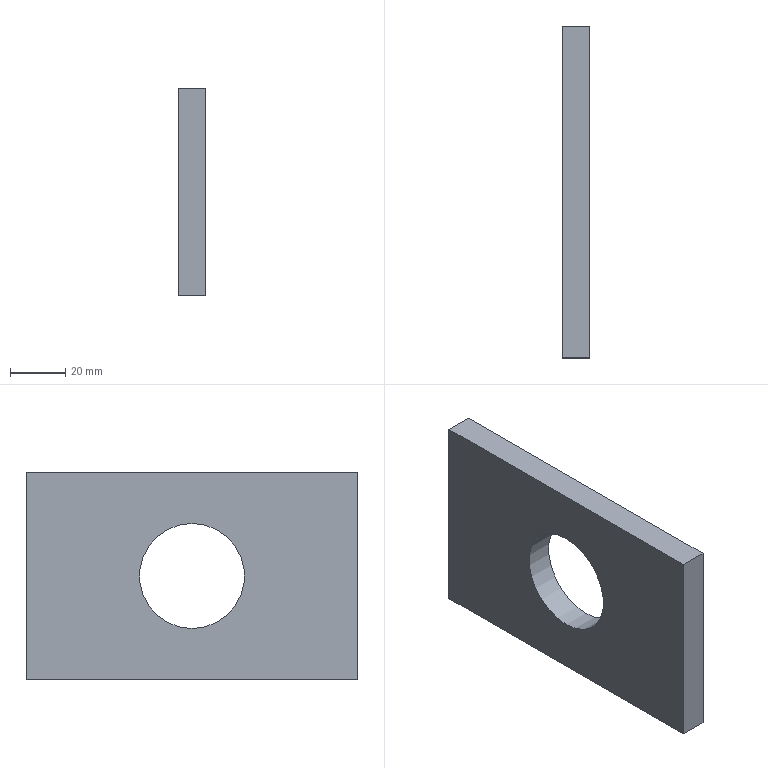Part | STEP file | Tube feed_id386_x_t | 1 solid | 7 faces | box 10 x 120 x 75 mm | volume 78659 mm3 | plane 6 | cylinder 1 | commonest cylinder face diameters 38 x1
STEP:
#1=CARTESIAN_POINT('',(0.,0.,0.));
#2=DIRECTION('',(0.,0.,1.));
#3=DIRECTION('',(1.,0.,0.));
#4=AXIS2_PLACEMENT_3D('',#1,#2,#3);
#5=CARTESIAN_POINT('',(476.,471.936,-6.));
#6=VERTEX_POINT('',#5);
#7=CARTESIAN_POINT('',(476.,351.936,-6.));
#8=VERTEX_POINT('',#7);
#9=CARTESIAN_POINT('',(476.,471.936,-6.));
#10=DIRECTION('',(0.,-1.,0.));
#11=VECTOR('',#10,1.);
#12=LINE('',#9,#11);
#13=CARTESIAN_POINT('',(476.,0.,0.));
#14=DIRECTION('',(1.,0.,0.));
#15=DIRECTION('',(0.,0.,-1.));
#16=AXIS2_PLACEMENT_3D('',#13,#14,#15);
#17=PLANE('',#16);
#18=CARTESIAN_POINT('',(6.,471.936));
#19=DIRECTION('',(0.,-1.));
#20=VECTOR('',#19,1.);
#21=LINE('',#18,#20);
#22=(GEOMETRIC_REPRESENTATION_CONTEXT(2)PARAMETRIC_REPRESENTATION_CONTEXT()REPRESENTATION_CONTEXT('',''));
#23=DEFINITIONAL_REPRESENTATION('',(#21),#22);
#24=PCURVE('',#17,#23);
#25=CARTESIAN_POINT('',(466.,471.936,-6.));
#26=DIRECTION('',(0.,0.,1.));
#27=DIRECTION('',(1.,0.,0.));
#28=AXIS2_PLACEMENT_3D('',#25,#26,#27);
#29=PLANE('',#28);
#30=CARTESIAN_POINT('',(10.,0.));
#31=DIRECTION('',(0.,-1.));
#32=VECTOR('',#31,1.);
#33=LINE('',#30,#32);
#34=(GEOMETRIC_REPRESENTATION_CONTEXT(2)PARAMETRIC_REPRESENTATION_CONTEXT()REPRESENTATION_CONTEXT('',''));
#35=DEFINITIONAL_REPRESENTATION('',(#33),#34);
#36=PCURVE('',#29,#35);
#37=SURFACE_CURVE('',#12,(#24,#36),.PCURVE_S1.);
#38=EDGE_CURVE('',#6,#8,#37,.T.);
#39=ORIENTED_EDGE('',*,*,#38,.T.);
#40=CARTESIAN_POINT('',(476.,351.936,-81.));
#41=VERTEX_POINT('',#40);
#42=CARTESIAN_POINT('',(476.,351.936,-6.));
#43=DIRECTION('',(0.,0.,-1.));
#44=VECTOR('',#43,1.);
#45=LINE('',#42,#44);
#46=CARTESIAN_POINT('',(6.,351.936));
#47=DIRECTION('',(1.,0.));
#48=VECTOR('',#47,1.);
#49=LINE('',#46,#48);
#50=(GEOMETRIC_REPRESENTATION_CONTEXT(2)PARAMETRIC_REPRESENTATION_CONTEXT()REPRESENTATION_CONTEXT('',''));
#51=DEFINITIONAL_REPRESENTATION('',(#49),#50);
#52=PCURVE('',#17,#51);
#53=CARTESIAN_POINT('',(466.,351.936,-6.));
#54=DIRECTION('',(0.,-1.,0.));
#55=DIRECTION('',(0.,0.,-1.));
#56=AXIS2_PLACEMENT_3D('',#53,#54,#55);
#57=PLANE('',#56);
#58=CARTESIAN_POINT('',(0.,10.));
#59=DIRECTION('',(1.,0.));
#60=VECTOR('',#59,1.);
#61=LINE('',#58,#60);
#62=(GEOMETRIC_REPRESENTATION_CONTEXT(2)PARAMETRIC_REPRESENTATION_CONTEXT()REPRESENTATION_CONTEXT('',''));
#63=DEFINITIONAL_REPRESENTATION('',(#61),#62);
#64=PCURVE('',#57,#63);
#65=SURFACE_CURVE('',#45,(#52,#64),.PCURVE_S1.);
#66=EDGE_CURVE('',#8,#41,#65,.T.);
#67=ORIENTED_EDGE('',*,*,#66,.T.);
#68=CARTESIAN_POINT('',(476.,471.936,-81.));
#69=VERTEX_POINT('',#68);
#70=CARTESIAN_POINT('',(476.,351.936,-81.));
#71=DIRECTION('',(0.,1.,0.));
#72=VECTOR('',#71,1.);
#73=LINE('',#70,#72);
#74=CARTESIAN_POINT('',(81.,351.936));
#75=DIRECTION('',(0.,1.));
#76=VECTOR('',#75,1.);
#77=LINE('',#74,#76);
#78=(GEOMETRIC_REPRESENTATION_CONTEXT(2)PARAMETRIC_REPRESENTATION_CONTEXT()REPRESENTATION_CONTEXT('',''));
#79=DEFINITIONAL_REPRESENTATION('',(#77),#78);
#80=PCURVE('',#17,#79);
#81=CARTESIAN_POINT('',(466.,351.936,-81.));
#82=DIRECTION('',(0.,0.,-1.));
#83=DIRECTION('',(-1.,0.,0.));
#84=AXIS2_PLACEMENT_3D('',#81,#82,#83);
#85=PLANE('',#84);
#86=CARTESIAN_POINT('',(-10.,0.));
#87=DIRECTION('',(0.,1.));
#88=VECTOR('',#87,1.);
#89=LINE('',#86,#88);
#90=(GEOMETRIC_REPRESENTATION_CONTEXT(2)PARAMETRIC_REPRESENTATION_CONTEXT()REPRESENTATION_CONTEXT('',''));
#91=DEFINITIONAL_REPRESENTATION('',(#89),#90);
#92=PCURVE('',#85,#91);
#93=SURFACE_CURVE('',#73,(#80,#92),.PCURVE_S1.);
#94=EDGE_CURVE('',#41,#69,#93,.T.);
#95=ORIENTED_EDGE('',*,*,#94,.T.);
#96=CARTESIAN_POINT('',(476.,471.936,-81.));
#97=DIRECTION('',(0.,0.,1.));
#98=VECTOR('',#97,1.);
#99=LINE('',#96,#98);
#100=CARTESIAN_POINT('',(81.,471.936));
#101=DIRECTION('',(-1.,0.));
#102=VECTOR('',#101,1.);
#103=LINE('',#100,#102);
#104=(GEOMETRIC_REPRESENTATION_CONTEXT(2)PARAMETRIC_REPRESENTATION_CONTEXT()REPRESENTATION_CONTEXT('',''));
#105=DEFINITIONAL_REPRESENTATION('',(#103),#104);
#106=PCURVE('',#17,#105);
#107=CARTESIAN_POINT('',(466.,471.936,-81.));
#108=DIRECTION('',(0.,1.,0.));
#109=DIRECTION('',(0.,0.,1.));
#110=AXIS2_PLACEMENT_3D('',#107,#108,#109);
#111=PLANE('',#110);
#112=CARTESIAN_POINT('',(0.,10.));
#113=DIRECTION('',(1.,0.));
#114=VECTOR('',#113,1.);
#115=LINE('',#112,#114);
#116=(GEOMETRIC_REPRESENTATION_CONTEXT(2)PARAMETRIC_REPRESENTATION_CONTEXT()REPRESENTATION_CONTEXT('',''));
#117=DEFINITIONAL_REPRESENTATION('',(#115),#116);
#118=PCURVE('',#111,#117);
#119=SURFACE_CURVE('',#99,(#106,#118),.PCURVE_S1.);
#120=EDGE_CURVE('',#69,#6,#119,.T.);
#121=ORIENTED_EDGE('',*,*,#120,.T.);
#122=EDGE_LOOP('',(#39,#67,#95,#121));
#123=FACE_BOUND('',#122,.T.);
#124=CARTESIAN_POINT('',(476.,411.936,-62.5));
#125=VERTEX_POINT('',#124);
#126=CARTESIAN_POINT('',(476.,411.936,-43.5));
#127=DIRECTION('',(-1.,0.,0.));
#128=DIRECTION('',(0.,0.,-1.));
#129=AXIS2_PLACEMENT_3D('',#126,#127,#128);
#130=CIRCLE('',#129,19.);
#131=CARTESIAN_POINT('',(62.5,411.936));
#132=CARTESIAN_POINT('',(62.5,379.027));
#133=CARTESIAN_POINT('',(34.,395.481));
#134=CARTESIAN_POINT('',(5.5,411.936));
#135=CARTESIAN_POINT('',(34.,428.39));
#136=CARTESIAN_POINT('',(62.5,444.845));
#137=CARTESIAN_POINT('',(62.5,411.936));
#138=(BOUNDED_CURVE()B_SPLINE_CURVE(2,(#131,#132,#133,#134,#135,#136,#137),.UNSPECIFIED.,.T.,.F.)B_SPLINE_CURVE_WITH_KNOTS((1,2,2,2,2,1),(-2.094,0.,2.094,4.189,6.283,8.378),.UNSPECIFIED.)CURVE()GEOMETRIC_REPRESENTATION_ITEM()RATIONAL_B_SPLINE_CURVE((1.,0.5,1.,0.5,1.,0.5,1.))REPRESENTATION_ITEM(''));
#139=(GEOMETRIC_REPRESENTATION_CONTEXT(2)PARAMETRIC_REPRESENTATION_CONTEXT()REPRESENTATION_CONTEXT('',''));
#140=DEFINITIONAL_REPRESENTATION('',(#138),#139);
#141=PCURVE('',#17,#140);
#142=CARTESIAN_POINT('',(398.5,411.936,-43.5));
#143=DIRECTION('',(1.,0.,0.));
#144=DIRECTION('',(0.,0.,-1.));
#145=AXIS2_PLACEMENT_3D('',#142,#143,#144);
#146=CYLINDRICAL_SURFACE('',#145,19.);
#147=CARTESIAN_POINT('',(6.283,77.5));
#148=DIRECTION('',(-1.,0.));
#149=VECTOR('',#148,1.);
#150=LINE('',#147,#149);
#151=(GEOMETRIC_REPRESENTATION_CONTEXT(2)PARAMETRIC_REPRESENTATION_CONTEXT()REPRESENTATION_CONTEXT('',''));
#152=DEFINITIONAL_REPRESENTATION('',(#150),#151);
#153=PCURVE('',#146,#152);
#154=SURFACE_CURVE('',#130,(#141,#153),.PCURVE_S1.);
#155=EDGE_CURVE('',#125,#125,#154,.T.);
#156=ORIENTED_EDGE('',*,*,#155,.T.);
#157=EDGE_LOOP('',(#156));
#158=FACE_BOUND('',#157,.T.);
#159=ADVANCED_FACE('',(#123,#158),#17,.T.);
#160=ORIENTED_EDGE('',*,*,#66,.F.);
#161=CARTESIAN_POINT('',(466.,351.936,-6.));
#162=VERTEX_POINT('',#161);
#163=CARTESIAN_POINT('',(466.,351.936,-6.));
#164=DIRECTION('',(1.,0.,0.));
#165=VECTOR('',#164,1.);
#166=LINE('',#163,#165);
#167=CARTESIAN_POINT('',(0.,0.));
#168=DIRECTION('',(0.,1.));
#169=VECTOR('',#168,1.);
#170=LINE('',#167,#169);
#171=(GEOMETRIC_REPRESENTATION_CONTEXT(2)PARAMETRIC_REPRESENTATION_CONTEXT()REPRESENTATION_CONTEXT('',''));
#172=DEFINITIONAL_REPRESENTATION('',(#170),#171);
#173=PCURVE('',#57,#172);
#174=CARTESIAN_POINT('',(0.,-120.));
#175=DIRECTION('',(1.,0.));
#176=VECTOR('',#175,1.);
#177=LINE('',#174,#176);
#178=(GEOMETRIC_REPRESENTATION_CONTEXT(2)PARAMETRIC_REPRESENTATION_CONTEXT()REPRESENTATION_CONTEXT('',''));
#179=DEFINITIONAL_REPRESENTATION('',(#177),#178);
#180=PCURVE('',#29,#179);
#181=SURFACE_CURVE('',#166,(#173,#180),.PCURVE_S1.);
#182=EDGE_CURVE('',#162,#8,#181,.T.);
#183=ORIENTED_EDGE('',*,*,#182,.F.);
#184=CARTESIAN_POINT('',(466.,351.936,-81.));
#185=VERTEX_POINT('',#184);
#186=CARTESIAN_POINT('',(466.,351.936,-6.));
#187=DIRECTION('',(0.,0.,-1.));
#188=VECTOR('',#187,1.);
#189=LINE('',#186,#188);
#190=CARTESIAN_POINT('',(0.,0.));
#191=DIRECTION('',(1.,0.));
#192=VECTOR('',#191,1.);
#193=LINE('',#190,#192);
#194=(GEOMETRIC_REPRESENTATION_CONTEXT(2)PARAMETRIC_REPRESENTATION_CONTEXT()REPRESENTATION_CONTEXT('',''));
#195=DEFINITIONAL_REPRESENTATION('',(#193),#194);
#196=PCURVE('',#57,#195);
#197=CARTESIAN_POINT('',(466.,0.,0.));
#198=DIRECTION('',(1.,0.,0.));
#199=DIRECTION('',(0.,0.,-1.));
#200=AXIS2_PLACEMENT_3D('',#197,#198,#199);
#201=PLANE('',#200);
#202=CARTESIAN_POINT('',(6.,351.936));
#203=DIRECTION('',(1.,0.));
#204=VECTOR('',#203,1.);
#205=LINE('',#202,#204);
#206=(GEOMETRIC_REPRESENTATION_CONTEXT(2)PARAMETRIC_REPRESENTATION_CONTEXT()REPRESENTATION_CONTEXT('',''));
#207=DEFINITIONAL_REPRESENTATION('',(#205),#206);
#208=PCURVE('',#201,#207);
#209=SURFACE_CURVE('',#189,(#196,#208),.PCURVE_S1.);
#210=EDGE_CURVE('',#162,#185,#209,.T.);
#211=ORIENTED_EDGE('',*,*,#210,.T.);
#212=CARTESIAN_POINT('',(466.,351.936,-81.));
#213=DIRECTION('',(1.,0.,0.));
#214=VECTOR('',#213,1.);
#215=LINE('',#212,#214);
#216=CARTESIAN_POINT('',(75.,0.));
#217=DIRECTION('',(0.,1.));
#218=VECTOR('',#217,1.);
#219=LINE('',#216,#218);
#220=(GEOMETRIC_REPRESENTATION_CONTEXT(2)PARAMETRIC_REPRESENTATION_CONTEXT()REPRESENTATION_CONTEXT('',''));
#221=DEFINITIONAL_REPRESENTATION('',(#219),#220);
#222=PCURVE('',#57,#221);
#223=CARTESIAN_POINT('',(0.,0.));
#224=DIRECTION('',(-1.,0.));
#225=VECTOR('',#224,1.);
#226=LINE('',#223,#225);
#227=(GEOMETRIC_REPRESENTATION_CONTEXT(2)PARAMETRIC_REPRESENTATION_CONTEXT()REPRESENTATION_CONTEXT('',''));
#228=DEFINITIONAL_REPRESENTATION('',(#226),#227);
#229=PCURVE('',#85,#228);
#230=SURFACE_CURVE('',#215,(#222,#229),.PCURVE_S1.);
#231=EDGE_CURVE('',#185,#41,#230,.T.);
#232=ORIENTED_EDGE('',*,*,#231,.T.);
#233=EDGE_LOOP('',(#160,#183,#211,#232));
#234=FACE_BOUND('',#233,.T.);
#235=ADVANCED_FACE('',(#234),#57,.T.);
#236=ORIENTED_EDGE('',*,*,#94,.F.);
#237=ORIENTED_EDGE('',*,*,#231,.F.);
#238=CARTESIAN_POINT('',(466.,471.936,-81.));
#239=VERTEX_POINT('',#238);
#240=CARTESIAN_POINT('',(466.,351.936,-81.));
#241=DIRECTION('',(0.,1.,0.));
#242=VECTOR('',#241,1.);
#243=LINE('',#240,#242);
#244=CARTESIAN_POINT('',(0.,0.));
#245=DIRECTION('',(0.,1.));
#246=VECTOR('',#245,1.);
#247=LINE('',#244,#246);
#248=(GEOMETRIC_REPRESENTATION_CONTEXT(2)PARAMETRIC_REPRESENTATION_CONTEXT()REPRESENTATION_CONTEXT('',''));
#249=DEFINITIONAL_REPRESENTATION('',(#247),#248);
#250=PCURVE('',#85,#249);
#251=CARTESIAN_POINT('',(81.,351.936));
#252=DIRECTION('',(0.,1.));
#253=VECTOR('',#252,1.);
#254=LINE('',#251,#253);
#255=(GEOMETRIC_REPRESENTATION_CONTEXT(2)PARAMETRIC_REPRESENTATION_CONTEXT()REPRESENTATION_CONTEXT('',''));
#256=DEFINITIONAL_REPRESENTATION('',(#254),#255);
#257=PCURVE('',#201,#256);
#258=SURFACE_CURVE('',#243,(#250,#257),.PCURVE_S1.);
#259=EDGE_CURVE('',#185,#239,#258,.T.);
#260=ORIENTED_EDGE('',*,*,#259,.T.);
#261=CARTESIAN_POINT('',(466.,471.936,-81.));
#262=DIRECTION('',(1.,0.,0.));
#263=VECTOR('',#262,1.);
#264=LINE('',#261,#263);
#265=CARTESIAN_POINT('',(0.,120.));
#266=DIRECTION('',(-1.,0.));
#267=VECTOR('',#266,1.);
#268=LINE('',#265,#267);
#269=(GEOMETRIC_REPRESENTATION_CONTEXT(2)PARAMETRIC_REPRESENTATION_CONTEXT()REPRESENTATION_CONTEXT('',''));
#270=DEFINITIONAL_REPRESENTATION('',(#268),#269);
#271=PCURVE('',#85,#270);
#272=CARTESIAN_POINT('',(0.,0.));
#273=DIRECTION('',(0.,1.));
#274=VECTOR('',#273,1.);
#275=LINE('',#272,#274);
#276=(GEOMETRIC_REPRESENTATION_CONTEXT(2)PARAMETRIC_REPRESENTATION_CONTEXT()REPRESENTATION_CONTEXT('',''));
#277=DEFINITIONAL_REPRESENTATION('',(#275),#276);
#278=PCURVE('',#111,#277);
#279=SURFACE_CURVE('',#264,(#271,#278),.PCURVE_S1.);
#280=EDGE_CURVE('',#239,#69,#279,.T.);
#281=ORIENTED_EDGE('',*,*,#280,.T.);
#282=EDGE_LOOP('',(#236,#237,#260,#281));
#283=FACE_BOUND('',#282,.T.);
#284=ADVANCED_FACE('',(#283),#85,.T.);
#285=ORIENTED_EDGE('',*,*,#120,.F.);
#286=ORIENTED_EDGE('',*,*,#280,.F.);
#287=CARTESIAN_POINT('',(466.,471.936,-6.));
#288=VERTEX_POINT('',#287);
#289=CARTESIAN_POINT('',(466.,471.936,-81.));
#290=DIRECTION('',(0.,0.,1.));
#291=VECTOR('',#290,1.);
#292=LINE('',#289,#291);
#293=CARTESIAN_POINT('',(0.,0.));
#294=DIRECTION('',(1.,0.));
#295=VECTOR('',#294,1.);
#296=LINE('',#293,#295);
#297=(GEOMETRIC_REPRESENTATION_CONTEXT(2)PARAMETRIC_REPRESENTATION_CONTEXT()REPRESENTATION_CONTEXT('',''));
#298=DEFINITIONAL_REPRESENTATION('',(#296),#297);
#299=PCURVE('',#111,#298);
#300=CARTESIAN_POINT('',(81.,471.936));
#301=DIRECTION('',(-1.,0.));
#302=VECTOR('',#301,1.);
#303=LINE('',#300,#302);
#304=(GEOMETRIC_REPRESENTATION_CONTEXT(2)PARAMETRIC_REPRESENTATION_CONTEXT()REPRESENTATION_CONTEXT('',''));
#305=DEFINITIONAL_REPRESENTATION('',(#303),#304);
#306=PCURVE('',#201,#305);
#307=SURFACE_CURVE('',#292,(#299,#306),.PCURVE_S1.);
#308=EDGE_CURVE('',#239,#288,#307,.T.);
#309=ORIENTED_EDGE('',*,*,#308,.T.);
#310=CARTESIAN_POINT('',(466.,471.936,-6.));
#311=DIRECTION('',(1.,0.,0.));
#312=VECTOR('',#311,1.);
#313=LINE('',#310,#312);
#314=CARTESIAN_POINT('',(75.,0.));
#315=DIRECTION('',(0.,1.));
#316=VECTOR('',#315,1.);
#317=LINE('',#314,#316);
#318=(GEOMETRIC_REPRESENTATION_CONTEXT(2)PARAMETRIC_REPRESENTATION_CONTEXT()REPRESENTATION_CONTEXT('',''));
#319=DEFINITIONAL_REPRESENTATION('',(#317),#318);
#320=PCURVE('',#111,#319);
#321=CARTESIAN_POINT('',(0.,0.));
#322=DIRECTION('',(1.,0.));
#323=VECTOR('',#322,1.);
#324=LINE('',#321,#323);
#325=(GEOMETRIC_REPRESENTATION_CONTEXT(2)PARAMETRIC_REPRESENTATION_CONTEXT()REPRESENTATION_CONTEXT('',''));
#326=DEFINITIONAL_REPRESENTATION('',(#324),#325);
#327=PCURVE('',#29,#326);
#328=SURFACE_CURVE('',#313,(#320,#327),.PCURVE_S1.);
#329=EDGE_CURVE('',#288,#6,#328,.T.);
#330=ORIENTED_EDGE('',*,*,#329,.T.);
#331=EDGE_LOOP('',(#285,#286,#309,#330));
#332=FACE_BOUND('',#331,.T.);
#333=ADVANCED_FACE('',(#332),#111,.T.);
#334=ORIENTED_EDGE('',*,*,#38,.F.);
#335=ORIENTED_EDGE('',*,*,#329,.F.);
#336=CARTESIAN_POINT('',(466.,471.936,-6.));
#337=DIRECTION('',(0.,-1.,0.));
#338=VECTOR('',#337,1.);
#339=LINE('',#336,#338);
#340=CARTESIAN_POINT('',(0.,0.));
#341=DIRECTION('',(0.,-1.));
#342=VECTOR('',#341,1.);
#343=LINE('',#340,#342);
#344=(GEOMETRIC_REPRESENTATION_CONTEXT(2)PARAMETRIC_REPRESENTATION_CONTEXT()REPRESENTATION_CONTEXT('',''));
#345=DEFINITIONAL_REPRESENTATION('',(#343),#344);
#346=PCURVE('',#29,#345);
#347=CARTESIAN_POINT('',(6.,471.936));
#348=DIRECTION('',(0.,-1.));
#349=VECTOR('',#348,1.);
#350=LINE('',#347,#349);
#351=(GEOMETRIC_REPRESENTATION_CONTEXT(2)PARAMETRIC_REPRESENTATION_CONTEXT()REPRESENTATION_CONTEXT('',''));
#352=DEFINITIONAL_REPRESENTATION('',(#350),#351);
#353=PCURVE('',#201,#352);
#354=SURFACE_CURVE('',#339,(#346,#353),.PCURVE_S1.);
#355=EDGE_CURVE('',#288,#162,#354,.T.);
#356=ORIENTED_EDGE('',*,*,#355,.T.);
#357=ORIENTED_EDGE('',*,*,#182,.T.);
#358=EDGE_LOOP('',(#334,#335,#356,#357));
#359=FACE_BOUND('',#358,.T.);
#360=ADVANCED_FACE('',(#359),#29,.T.);
#361=CARTESIAN_POINT('',(466.,411.936,-62.5));
#362=VERTEX_POINT('',#361);
#363=CARTESIAN_POINT('',(466.,411.936,-43.5));
#364=DIRECTION('',(-1.,0.,0.));
#365=DIRECTION('',(0.,0.,-1.));
#366=AXIS2_PLACEMENT_3D('',#363,#364,#365);
#367=CIRCLE('',#366,19.);
#368=CARTESIAN_POINT('',(62.5,411.936));
#369=CARTESIAN_POINT('',(62.5,379.027));
#370=CARTESIAN_POINT('',(34.,395.481));
#371=CARTESIAN_POINT('',(5.5,411.936));
#372=CARTESIAN_POINT('',(34.,428.39));
#373=CARTESIAN_POINT('',(62.5,444.845));
#374=CARTESIAN_POINT('',(62.5,411.936));
#375=(BOUNDED_CURVE()B_SPLINE_CURVE(2,(#368,#369,#370,#371,#372,#373,#374),.UNSPECIFIED.,.T.,.F.)B_SPLINE_CURVE_WITH_KNOTS((1,2,2,2,2,1),(-2.094,0.,2.094,4.189,6.283,8.378),.UNSPECIFIED.)CURVE()GEOMETRIC_REPRESENTATION_ITEM()RATIONAL_B_SPLINE_CURVE((1.,0.5,1.,0.5,1.,0.5,1.))REPRESENTATION_ITEM(''));
#376=(GEOMETRIC_REPRESENTATION_CONTEXT(2)PARAMETRIC_REPRESENTATION_CONTEXT()REPRESENTATION_CONTEXT('',''));
#377=DEFINITIONAL_REPRESENTATION('',(#375),#376);
#378=PCURVE('',#201,#377);
#379=CARTESIAN_POINT('',(6.283,67.5));
#380=DIRECTION('',(-1.,0.));
#381=VECTOR('',#380,1.);
#382=LINE('',#379,#381);
#383=(GEOMETRIC_REPRESENTATION_CONTEXT(2)PARAMETRIC_REPRESENTATION_CONTEXT()REPRESENTATION_CONTEXT('',''));
#384=DEFINITIONAL_REPRESENTATION('',(#382),#383);
#385=PCURVE('',#146,#384);
#386=SURFACE_CURVE('',#367,(#378,#385),.PCURVE_S1.);
#387=EDGE_CURVE('',#362,#362,#386,.T.);
#388=ORIENTED_EDGE('',*,*,#387,.F.);
#389=EDGE_LOOP('',(#388));
#390=FACE_BOUND('',#389,.T.);
#391=ORIENTED_EDGE('',*,*,#210,.F.);
#392=ORIENTED_EDGE('',*,*,#355,.F.);
#393=ORIENTED_EDGE('',*,*,#308,.F.);
#394=ORIENTED_EDGE('',*,*,#259,.F.);
#395=EDGE_LOOP('',(#391,#392,#393,#394));
#396=FACE_BOUND('',#395,.T.);
#397=ADVANCED_FACE('',(#390,#396),#201,.F.);
#398=ORIENTED_EDGE('',*,*,#155,.T.);
#399=CARTESIAN_POINT('',(466.,411.936,-62.5));
#400=CARTESIAN_POINT('',(476.,411.936,-62.5));
#401=B_SPLINE_CURVE_WITH_KNOTS('',1,(#399,#400),.UNSPECIFIED.,.F.,.F.,(2,2),(67.5,77.5),.PIECEWISE_BEZIER_KNOTS.);
#402=CARTESIAN_POINT('',(0.,0.));
#403=DIRECTION('',(0.,1.));
#404=VECTOR('',#403,1.);
#405=LINE('',#402,#404);
#406=(GEOMETRIC_REPRESENTATION_CONTEXT(2)PARAMETRIC_REPRESENTATION_CONTEXT()REPRESENTATION_CONTEXT('',''));
#407=DEFINITIONAL_REPRESENTATION('',(#405),#406);
#408=PCURVE('',#146,#407);
#409=CARTESIAN_POINT('',(6.283,0.));
#410=DIRECTION('',(0.,1.));
#411=VECTOR('',#410,1.);
#412=LINE('',#409,#411);
#413=(GEOMETRIC_REPRESENTATION_CONTEXT(2)PARAMETRIC_REPRESENTATION_CONTEXT()REPRESENTATION_CONTEXT('',''));
#414=DEFINITIONAL_REPRESENTATION('',(#412),#413);
#415=PCURVE('',#146,#414);
#416=SEAM_CURVE('',#401,(#408,#415),.PCURVE_S1.);
#417=EDGE_CURVE('',#362,#125,#416,.T.);
#418=ORIENTED_EDGE('',*,*,#417,.F.);
#419=ORIENTED_EDGE('',*,*,#387,.F.);
#420=ORIENTED_EDGE('',*,*,#417,.T.);
#421=EDGE_LOOP('',(#398,#418,#419,#420));
#422=FACE_BOUND('',#421,.F.);
#423=ADVANCED_FACE('',(#422),#146,.F.);
#424=CLOSED_SHELL('',(#159,#235,#284,#333,#360,#397,#423));
#425=MANIFOLD_SOLID_BREP('',#424);
#426=(LENGTH_UNIT()NAMED_UNIT(*)SI_UNIT(.MILLI.,.METRE.));
#427=UNCERTAINTY_MEASURE_WITH_UNIT(LENGTH_MEASURE(0.000002),#426,'','');
#428=(NAMED_UNIT(*)PLANE_ANGLE_UNIT()SI_UNIT($,.RADIAN.));
#429=(NAMED_UNIT(*)SI_UNIT($,.STERADIAN.)SOLID_ANGLE_UNIT());
#430=(GEOMETRIC_REPRESENTATION_CONTEXT(3)GLOBAL_UNCERTAINTY_ASSIGNED_CONTEXT((#427))GLOBAL_UNIT_ASSIGNED_CONTEXT((#426,#428,#429))REPRESENTATION_CONTEXT('',''));
#431=ADVANCED_BREP_SHAPE_REPRESENTATION('',(#4,#425),#430);